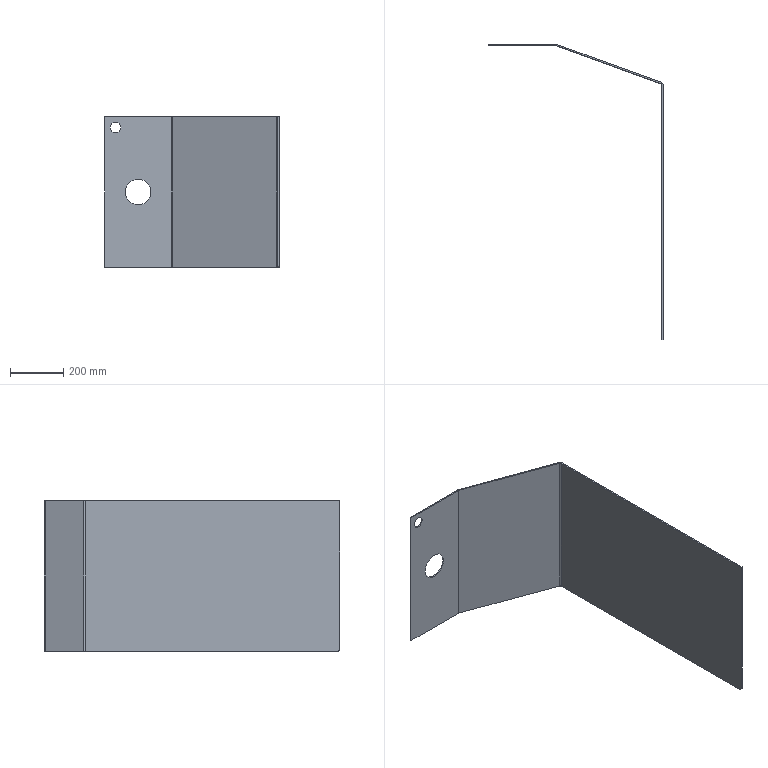Part | SolidWorks | features Fillet 1, FlatPattern 1, ICE 1, SMBaseFlange 1, SheetMetal 1, UnFold 1 | 1 solid | 27 faces | box 655 x 1110 x 565 mm | volume 4586470 mm3 | plane 18 | cylinder 9 | commonest cylinder face diameters 12 x2 22 x2 40 x2 97 x2 14 x1
STEP:
#1=CARTESIAN_POINT('',(125.,1105.,-48.5));
#2=VERTEX_POINT('',#1);
#3=CARTESIAN_POINT('',(125.,1105.,48.5));
#4=VERTEX_POINT('',#3);
#5=CARTESIAN_POINT('',(125.,1105.,0.));
#6=DIRECTION('',(0.,1.,0.));
#7=DIRECTION('',(0.,0.,1.));
#8=AXIS2_PLACEMENT_3D('',#5,#6,#7);
#9=CIRCLE('',#8,48.5);
#10=EDGE_CURVE('',#2,#4,#9,.T.);
#11=ORIENTED_EDGE('',*,*,#10,.F.);
#12=CARTESIAN_POINT('',(125.,1110.,-48.5));
#13=VERTEX_POINT('',#12);
#14=CARTESIAN_POINT('',(125.,0.,-48.5));
#15=DIRECTION('',(0.,1.,0.));
#16=VECTOR('',#15,1000.);
#17=LINE('',#14,#16);
#18=EDGE_CURVE('',#2,#13,#17,.T.);
#19=ORIENTED_EDGE('',*,*,#18,.T.);
#20=CARTESIAN_POINT('',(125.,1110.,48.5));
#21=VERTEX_POINT('',#20);
#22=CARTESIAN_POINT('',(125.,1110.,0.));
#23=DIRECTION('',(0.,1.,0.));
#24=DIRECTION('',(0.,0.,1.));
#25=AXIS2_PLACEMENT_3D('',#22,#23,#24);
#26=CIRCLE('',#25,48.5);
#27=EDGE_CURVE('',#13,#21,#26,.T.);
#28=ORIENTED_EDGE('',*,*,#27,.T.);
#29=CARTESIAN_POINT('',(125.,0.,48.5));
#30=DIRECTION('',(0.,1.,0.));
#31=VECTOR('',#30,1000.);
#32=LINE('',#29,#31);
#33=EDGE_CURVE('',#4,#21,#32,.T.);
#34=ORIENTED_EDGE('',*,*,#33,.F.);
#35=EDGE_LOOP('',(#11,#19,#28,#34));
#36=FACE_OUTER_BOUND('',#35,.T.);
#37=CARTESIAN_POINT('',(125.,0.,0.));
#38=DIRECTION('',(0.,1.,0.));
#39=DIRECTION('',(0.,0.,1.));
#40=AXIS2_PLACEMENT_3D('',#37,#38,#39);
#41=CYLINDRICAL_SURFACE('',#40,48.5);
#42=ADVANCED_FACE('',(#36),#41,.F.);
#43=CARTESIAN_POINT('',(40.,1105.,222.5));
#44=VERTEX_POINT('',#43);
#45=CARTESIAN_POINT('',(40.,1105.,262.5));
#46=VERTEX_POINT('',#45);
#47=CARTESIAN_POINT('',(40.,1105.,242.5));
#48=DIRECTION('',(0.,1.,0.));
#49=DIRECTION('',(0.,0.,1.));
#50=AXIS2_PLACEMENT_3D('',#47,#48,#49);
#51=CIRCLE('',#50,20.);
#52=EDGE_CURVE('',#44,#46,#51,.T.);
#53=ORIENTED_EDGE('',*,*,#52,.F.);
#54=CARTESIAN_POINT('',(40.,1110.,222.5));
#55=VERTEX_POINT('',#54);
#56=CARTESIAN_POINT('',(40.,0.,222.5));
#57=DIRECTION('',(0.,1.,0.));
#58=VECTOR('',#57,1000.);
#59=LINE('',#56,#58);
#60=EDGE_CURVE('',#44,#55,#59,.T.);
#61=ORIENTED_EDGE('',*,*,#60,.T.);
#62=CARTESIAN_POINT('',(40.,1110.,262.5));
#63=VERTEX_POINT('',#62);
#64=CARTESIAN_POINT('',(40.,1110.,242.5));
#65=DIRECTION('',(0.,1.,0.));
#66=DIRECTION('',(0.,0.,1.));
#67=AXIS2_PLACEMENT_3D('',#64,#65,#66);
#68=CIRCLE('',#67,20.);
#69=EDGE_CURVE('',#55,#63,#68,.T.);
#70=ORIENTED_EDGE('',*,*,#69,.T.);
#71=CARTESIAN_POINT('',(40.,0.,262.5));
#72=DIRECTION('',(0.,1.,0.));
#73=VECTOR('',#72,1000.);
#74=LINE('',#71,#73);
#75=EDGE_CURVE('',#46,#63,#74,.T.);
#76=ORIENTED_EDGE('',*,*,#75,.F.);
#77=EDGE_LOOP('',(#53,#61,#70,#76));
#78=FACE_OUTER_BOUND('',#77,.T.);
#79=CARTESIAN_POINT('',(40.,0.,242.5));
#80=DIRECTION('',(0.,1.,0.));
#81=DIRECTION('',(0.,0.,1.));
#82=AXIS2_PLACEMENT_3D('',#79,#80,#81);
#83=CYLINDRICAL_SURFACE('',#82,20.);
#84=ADVANCED_FACE('',(#78),#83,.F.);
#85=CARTESIAN_POINT('',(255.823,1109.337,282.5));
#86=VERTEX_POINT('',#85);
#87=CARTESIAN_POINT('',(254.113,1104.638,282.5));
#88=VERTEX_POINT('',#87);
#89=CARTESIAN_POINT('',(255.823,1109.337,282.5));
#90=DIRECTION('',(-0.342,-0.9397,0.));
#91=VECTOR('',#90,1000.);
#92=LINE('',#89,#91);
#93=EDGE_CURVE('',#86,#88,#92,.T.);
#94=ORIENTED_EDGE('',*,*,#93,.F.);
#95=CARTESIAN_POINT('',(252.06,1110.,282.5));
#96=VERTEX_POINT('',#95);
#97=CARTESIAN_POINT('',(252.06,1099.,282.5));
#98=DIRECTION('',(0.,0.,-1.));
#99=DIRECTION('',(1.,0.,0.));
#100=AXIS2_PLACEMENT_3D('',#97,#98,#99);
#101=CIRCLE('',#100,11.);
#102=EDGE_CURVE('',#96,#86,#101,.T.);
#103=ORIENTED_EDGE('',*,*,#102,.F.);
#104=CARTESIAN_POINT('',(252.06,1105.,282.5));
#105=VERTEX_POINT('',#104);
#106=CARTESIAN_POINT('',(252.06,1105.,282.5));
#107=DIRECTION('',(0.,1.,0.));
#108=VECTOR('',#107,1000.);
#109=LINE('',#106,#108);
#110=EDGE_CURVE('',#105,#96,#109,.T.);
#111=ORIENTED_EDGE('',*,*,#110,.F.);
#112=CARTESIAN_POINT('',(252.06,1099.,282.5));
#113=DIRECTION('',(0.,0.,-1.));
#114=DIRECTION('',(1.,0.,0.));
#115=AXIS2_PLACEMENT_3D('',#112,#113,#114);
#116=CIRCLE('',#115,6.);
#117=EDGE_CURVE('',#105,#88,#116,.T.);
#118=ORIENTED_EDGE('',*,*,#117,.T.);
#119=EDGE_LOOP('',(#94,#103,#111,#118));
#120=FACE_OUTER_BOUND('',#119,.T.);
#121=CARTESIAN_POINT('',(255.823,1109.337,282.5));
#122=DIRECTION('',(0.,0.,1.));
#123=DIRECTION('',(1.,0.,0.));
#124=AXIS2_PLACEMENT_3D('',#121,#122,#123);
#125=PLANE('',#124);
#126=ADVANCED_FACE('',(#120),#125,.T.);
#127=CARTESIAN_POINT('',(647.762,966.682,282.5));
#128=VERTEX_POINT('',#127);
#129=CARTESIAN_POINT('',(254.,1110.,282.5));
#130=DIRECTION('',(0.9397,-0.342,0.));
#131=VECTOR('',#130,1000.);
#132=LINE('',#129,#131);
#133=EDGE_CURVE('',#86,#128,#132,.T.);
#134=ORIENTED_EDGE('',*,*,#133,.F.);
#135=ORIENTED_EDGE('',*,*,#93,.T.);
#136=CARTESIAN_POINT('',(646.052,961.984,282.5));
#137=VERTEX_POINT('',#136);
#138=CARTESIAN_POINT('',(252.29,1105.302,282.5));
#139=DIRECTION('',(0.9397,-0.342,0.));
#140=VECTOR('',#139,1000.);
#141=LINE('',#138,#140);
#142=EDGE_CURVE('',#88,#137,#141,.T.);
#143=ORIENTED_EDGE('',*,*,#142,.T.);
#144=CARTESIAN_POINT('',(646.052,961.984,282.5));
#145=DIRECTION('',(0.342,0.9397,0.));
#146=VECTOR('',#145,1000.);
#147=LINE('',#144,#146);
#148=EDGE_CURVE('',#137,#128,#147,.T.);
#149=ORIENTED_EDGE('',*,*,#148,.T.);
#150=EDGE_LOOP('',(#134,#135,#143,#149));
#151=FACE_OUTER_BOUND('',#150,.T.);
#152=CARTESIAN_POINT('',(252.06,1105.,282.5));
#153=DIRECTION('',(0.,0.,1.));
#154=DIRECTION('',(1.,0.,0.));
#155=AXIS2_PLACEMENT_3D('',#152,#153,#154);
#156=PLANE('',#155);
#157=ADVANCED_FACE('',(#151),#156,.T.);
#158=CARTESIAN_POINT('',(252.06,1110.,-282.5));
#159=VERTEX_POINT('',#158);
#160=CARTESIAN_POINT('',(252.06,1105.,-282.5));
#161=VERTEX_POINT('',#160);
#162=CARTESIAN_POINT('',(252.06,1110.,-282.5));
#163=DIRECTION('',(0.,-1.,0.));
#164=VECTOR('',#163,1000.);
#165=LINE('',#162,#164);
#166=EDGE_CURVE('',#159,#161,#165,.T.);
#167=ORIENTED_EDGE('',*,*,#166,.F.);
#168=CARTESIAN_POINT('',(255.823,1109.337,-282.5));
#169=VERTEX_POINT('',#168);
#170=CARTESIAN_POINT('',(252.06,1099.,-282.5));
#171=DIRECTION('',(0.,0.,-1.));
#172=DIRECTION('',(1.,0.,0.));
#173=AXIS2_PLACEMENT_3D('',#170,#171,#172);
#174=CIRCLE('',#173,11.);
#175=EDGE_CURVE('',#159,#169,#174,.T.);
#176=ORIENTED_EDGE('',*,*,#175,.T.);
#177=CARTESIAN_POINT('',(254.113,1104.638,-282.5));
#178=VERTEX_POINT('',#177);
#179=CARTESIAN_POINT('',(254.113,1104.638,-282.5));
#180=DIRECTION('',(0.342,0.9397,0.));
#181=VECTOR('',#180,1000.);
#182=LINE('',#179,#181);
#183=EDGE_CURVE('',#178,#169,#182,.T.);
#184=ORIENTED_EDGE('',*,*,#183,.F.);
#185=CARTESIAN_POINT('',(252.06,1099.,-282.5));
#186=DIRECTION('',(0.,0.,-1.));
#187=DIRECTION('',(1.,0.,0.));
#188=AXIS2_PLACEMENT_3D('',#185,#186,#187);
#189=CIRCLE('',#188,6.);
#190=EDGE_CURVE('',#161,#178,#189,.T.);
#191=ORIENTED_EDGE('',*,*,#190,.F.);
#192=EDGE_LOOP('',(#167,#176,#184,#191));
#193=FACE_OUTER_BOUND('',#192,.T.);
#194=CARTESIAN_POINT('',(252.06,1110.,-282.5));
#195=DIRECTION('',(0.,0.,-1.));
#196=DIRECTION('',(-1.,0.,0.));
#197=AXIS2_PLACEMENT_3D('',#194,#195,#196);
#198=PLANE('',#197);
#199=ADVANCED_FACE('',(#193),#198,.T.);
#200=CARTESIAN_POINT('',(0.,1110.,-282.5));
#201=VERTEX_POINT('',#200);
#202=CARTESIAN_POINT('',(0.,1110.,-282.5));
#203=DIRECTION('',(1.,0.,0.));
#204=VECTOR('',#203,1000.);
#205=LINE('',#202,#204);
#206=EDGE_CURVE('',#201,#159,#205,.T.);
#207=ORIENTED_EDGE('',*,*,#206,.T.);
#208=ORIENTED_EDGE('',*,*,#166,.T.);
#209=CARTESIAN_POINT('',(0.,1105.,-282.5));
#210=VERTEX_POINT('',#209);
#211=CARTESIAN_POINT('',(0.,1105.,-282.5));
#212=DIRECTION('',(1.,0.,0.));
#213=VECTOR('',#212,1000.);
#214=LINE('',#211,#213);
#215=EDGE_CURVE('',#210,#161,#214,.T.);
#216=ORIENTED_EDGE('',*,*,#215,.F.);
#217=CARTESIAN_POINT('',(0.,1105.,-282.5));
#218=DIRECTION('',(0.,1.,0.));
#219=VECTOR('',#218,1000.);
#220=LINE('',#217,#219);
#221=EDGE_CURVE('',#210,#201,#220,.T.);
#222=ORIENTED_EDGE('',*,*,#221,.T.);
#223=EDGE_LOOP('',(#207,#208,#216,#222));
#224=FACE_OUTER_BOUND('',#223,.T.);
#225=CARTESIAN_POINT('',(254.113,1104.638,-282.5));
#226=DIRECTION('',(0.,0.,-1.));
#227=DIRECTION('',(-1.,0.,0.));
#228=AXIS2_PLACEMENT_3D('',#225,#226,#227);
#229=PLANE('',#228);
#230=ADVANCED_FACE('',(#224),#229,.T.);
#231=CARTESIAN_POINT('',(655.,956.346,282.5));
#232=VERTEX_POINT('',#231);
#233=CARTESIAN_POINT('',(650.,956.346,282.5));
#234=VERTEX_POINT('',#233);
#235=CARTESIAN_POINT('',(655.,956.346,282.5));
#236=DIRECTION('',(-1.,0.,0.));
#237=VECTOR('',#236,1000.);
#238=LINE('',#235,#237);
#239=EDGE_CURVE('',#232,#234,#238,.T.);
#240=ORIENTED_EDGE('',*,*,#239,.F.);
#241=CARTESIAN_POINT('',(644.,956.346,282.5));
#242=DIRECTION('',(0.,0.,-1.));
#243=DIRECTION('',(1.,0.,0.));
#244=AXIS2_PLACEMENT_3D('',#241,#242,#243);
#245=CIRCLE('',#244,11.);
#246=EDGE_CURVE('',#128,#232,#245,.T.);
#247=ORIENTED_EDGE('',*,*,#246,.F.);
#248=ORIENTED_EDGE('',*,*,#148,.F.);
#249=CARTESIAN_POINT('',(644.,956.346,282.5));
#250=DIRECTION('',(0.,0.,-1.));
#251=DIRECTION('',(1.,0.,0.));
#252=AXIS2_PLACEMENT_3D('',#249,#250,#251);
#253=CIRCLE('',#252,6.);
#254=EDGE_CURVE('',#137,#234,#253,.T.);
#255=ORIENTED_EDGE('',*,*,#254,.T.);
#256=EDGE_LOOP('',(#240,#247,#248,#255));
#257=FACE_OUTER_BOUND('',#256,.T.);
#258=CARTESIAN_POINT('',(655.,956.346,282.5));
#259=DIRECTION('',(0.,0.,1.));
#260=DIRECTION('',(1.,0.,0.));
#261=AXIS2_PLACEMENT_3D('',#258,#259,#260);
#262=PLANE('',#261);
#263=ADVANCED_FACE('',(#257),#262,.T.);
#264=CARTESIAN_POINT('',(655.,0.,282.5));
#265=VERTEX_POINT('',#264);
#266=CARTESIAN_POINT('',(655.,964.048,282.5));
#267=DIRECTION('',(0.,-1.,0.));
#268=VECTOR('',#267,1000.);
#269=LINE('',#266,#268);
#270=EDGE_CURVE('',#232,#265,#269,.T.);
#271=ORIENTED_EDGE('',*,*,#270,.F.);
#272=ORIENTED_EDGE('',*,*,#239,.T.);
#273=CARTESIAN_POINT('',(650.,0.,282.5));
#274=VERTEX_POINT('',#273);
#275=CARTESIAN_POINT('',(650.,964.048,282.5));
#276=DIRECTION('',(0.,-1.,0.));
#277=VECTOR('',#276,1000.);
#278=LINE('',#275,#277);
#279=EDGE_CURVE('',#234,#274,#278,.T.);
#280=ORIENTED_EDGE('',*,*,#279,.T.);
#281=CARTESIAN_POINT('',(655.,0.,282.5));
#282=DIRECTION('',(-1.,0.,0.));
#283=VECTOR('',#282,1000.);
#284=LINE('',#281,#283);
#285=EDGE_CURVE('',#265,#274,#284,.T.);
#286=ORIENTED_EDGE('',*,*,#285,.F.);
#287=EDGE_LOOP('',(#271,#272,#280,#286));
#288=FACE_OUTER_BOUND('',#287,.T.);
#289=CARTESIAN_POINT('',(646.052,961.984,282.5));
#290=DIRECTION('',(0.,0.,1.));
#291=DIRECTION('',(1.,0.,0.));
#292=AXIS2_PLACEMENT_3D('',#289,#290,#291);
#293=PLANE('',#292);
#294=ADVANCED_FACE('',(#288),#293,.T.);
#295=CARTESIAN_POINT('',(647.762,966.682,-282.5));
#296=VERTEX_POINT('',#295);
#297=CARTESIAN_POINT('',(646.052,961.984,-282.5));
#298=VERTEX_POINT('',#297);
#299=CARTESIAN_POINT('',(647.762,966.682,-282.5));
#300=DIRECTION('',(-0.342,-0.9397,0.));
#301=VECTOR('',#300,1000.);
#302=LINE('',#299,#301);
#303=EDGE_CURVE('',#296,#298,#302,.T.);
#304=ORIENTED_EDGE('',*,*,#303,.F.);
#305=CARTESIAN_POINT('',(655.,956.346,-282.5));
#306=VERTEX_POINT('',#305);
#307=CARTESIAN_POINT('',(644.,956.346,-282.5));
#308=DIRECTION('',(0.,0.,-1.));
#309=DIRECTION('',(1.,0.,0.));
#310=AXIS2_PLACEMENT_3D('',#307,#308,#309);
#311=CIRCLE('',#310,11.);
#312=EDGE_CURVE('',#296,#306,#311,.T.);
#313=ORIENTED_EDGE('',*,*,#312,.T.);
#314=CARTESIAN_POINT('',(650.,956.346,-282.5));
#315=VERTEX_POINT('',#314);
#316=CARTESIAN_POINT('',(650.,956.346,-282.5));
#317=DIRECTION('',(1.,0.,0.));
#318=VECTOR('',#317,1000.);
#319=LINE('',#316,#318);
#320=EDGE_CURVE('',#315,#306,#319,.T.);
#321=ORIENTED_EDGE('',*,*,#320,.F.);
#322=CARTESIAN_POINT('',(644.,956.346,-282.5));
#323=DIRECTION('',(0.,0.,-1.));
#324=DIRECTION('',(1.,0.,0.));
#325=AXIS2_PLACEMENT_3D('',#322,#323,#324);
#326=CIRCLE('',#325,6.);
#327=EDGE_CURVE('',#298,#315,#326,.T.);
#328=ORIENTED_EDGE('',*,*,#327,.F.);
#329=EDGE_LOOP('',(#304,#313,#321,#328));
#330=FACE_OUTER_BOUND('',#329,.T.);
#331=CARTESIAN_POINT('',(647.762,966.682,-282.5));
#332=DIRECTION('',(0.,0.,-1.));
#333=DIRECTION('',(-1.,0.,0.));
#334=AXIS2_PLACEMENT_3D('',#331,#332,#333);
#335=PLANE('',#334);
#336=ADVANCED_FACE('',(#330),#335,.T.);
#337=CARTESIAN_POINT('',(254.,1110.,-282.5));
#338=DIRECTION('',(0.9397,-0.342,0.));
#339=VECTOR('',#338,1000.);
#340=LINE('',#337,#339);
#341=EDGE_CURVE('',#169,#296,#340,.T.);
#342=ORIENTED_EDGE('',*,*,#341,.T.);
#343=ORIENTED_EDGE('',*,*,#303,.T.);
#344=CARTESIAN_POINT('',(252.29,1105.302,-282.5));
#345=DIRECTION('',(0.9397,-0.342,0.));
#346=VECTOR('',#345,1000.);
#347=LINE('',#344,#346);
#348=EDGE_CURVE('',#178,#298,#347,.T.);
#349=ORIENTED_EDGE('',*,*,#348,.F.);
#350=ORIENTED_EDGE('',*,*,#183,.T.);
#351=EDGE_LOOP('',(#342,#343,#349,#350));
#352=FACE_OUTER_BOUND('',#351,.T.);
#353=CARTESIAN_POINT('',(650.,956.346,-282.5));
#354=DIRECTION('',(0.,0.,-1.));
#355=DIRECTION('',(-1.,0.,0.));
#356=AXIS2_PLACEMENT_3D('',#353,#354,#355);
#357=PLANE('',#356);
#358=ADVANCED_FACE('',(#352),#357,.T.);
#359=CARTESIAN_POINT('',(650.,7.,-282.5));
#360=VERTEX_POINT('',#359);
#361=CARTESIAN_POINT('',(650.,964.048,-282.5));
#362=DIRECTION('',(0.,-1.,0.));
#363=VECTOR('',#362,1000.);
#364=LINE('',#361,#363);
#365=EDGE_CURVE('',#315,#360,#364,.T.);
#366=ORIENTED_EDGE('',*,*,#365,.T.);
#367=CARTESIAN_POINT('',(650.,0.,-275.5));
#368=VERTEX_POINT('',#367);
#369=CARTESIAN_POINT('',(650.,7.,-275.5));
#370=DIRECTION('',(-1.,0.,0.));
#371=DIRECTION('',(0.,1.,0.));
#372=AXIS2_PLACEMENT_3D('',#369,#370,#371);
#373=CIRCLE('',#372,7.);
#374=EDGE_CURVE('',#360,#368,#373,.T.);
#375=ORIENTED_EDGE('',*,*,#374,.T.);
#376=CARTESIAN_POINT('',(650.,0.,282.5));
#377=DIRECTION('',(0.,0.,-1.));
#378=VECTOR('',#377,1000.);
#379=LINE('',#376,#378);
#380=EDGE_CURVE('',#274,#368,#379,.T.);
#381=ORIENTED_EDGE('',*,*,#380,.F.);
#382=ORIENTED_EDGE('',*,*,#279,.F.);
#383=CARTESIAN_POINT('',(650.,956.346,282.5));
#384=DIRECTION('',(0.,0.,-1.));
#385=VECTOR('',#384,1000.);
#386=LINE('',#383,#385);
#387=EDGE_CURVE('',#234,#315,#386,.T.);
#388=ORIENTED_EDGE('',*,*,#387,.T.);
#389=EDGE_LOOP('',(#366,#375,#381,#382,#388));
#390=FACE_OUTER_BOUND('',#389,.T.);
#391=CARTESIAN_POINT('',(650.,964.048,282.5));
#392=DIRECTION('',(1.,0.,0.));
#393=DIRECTION('',(0.,1.,0.));
#394=AXIS2_PLACEMENT_3D('',#391,#392,#393);
#395=PLANE('',#394);
#396=ADVANCED_FACE('',(#390),#395,.F.);
#397=ORIENTED_EDGE('',*,*,#380,.T.);
#398=CARTESIAN_POINT('',(655.,0.,-275.5));
#399=VERTEX_POINT('',#398);
#400=CARTESIAN_POINT('',(655.,0.,-275.5));
#401=DIRECTION('',(1.,0.,0.));
#402=VECTOR('',#401,1000.);
#403=LINE('',#400,#402);
#404=EDGE_CURVE('',#368,#399,#403,.T.);
#405=ORIENTED_EDGE('',*,*,#404,.T.);
#406=CARTESIAN_POINT('',(655.,0.,282.5));
#407=DIRECTION('',(0.,0.,-1.));
#408=VECTOR('',#407,1000.);
#409=LINE('',#406,#408);
#410=EDGE_CURVE('',#265,#399,#409,.T.);
#411=ORIENTED_EDGE('',*,*,#410,.F.);
#412=ORIENTED_EDGE('',*,*,#285,.T.);
#413=EDGE_LOOP('',(#397,#405,#411,#412));
#414=FACE_OUTER_BOUND('',#413,.T.);
#415=CARTESIAN_POINT('',(655.,0.,282.5));
#416=DIRECTION('',(0.,-1.,0.));
#417=DIRECTION('',(0.,0.,-1.));
#418=AXIS2_PLACEMENT_3D('',#415,#416,#417);
#419=PLANE('',#418);
#420=ADVANCED_FACE('',(#414),#419,.T.);
#421=ORIENTED_EDGE('',*,*,#410,.T.);
#422=CARTESIAN_POINT('',(655.,7.,-282.5));
#423=VERTEX_POINT('',#422);
#424=CARTESIAN_POINT('',(655.,7.,-275.5));
#425=DIRECTION('',(1.,0.,0.));
#426=DIRECTION('',(0.,1.,0.));
#427=AXIS2_PLACEMENT_3D('',#424,#425,#426);
#428=CIRCLE('',#427,7.);
#429=EDGE_CURVE('',#399,#423,#428,.T.);
#430=ORIENTED_EDGE('',*,*,#429,.T.);
#431=CARTESIAN_POINT('',(655.,964.048,-282.5));
#432=DIRECTION('',(0.,-1.,0.));
#433=VECTOR('',#432,1000.);
#434=LINE('',#431,#433);
#435=EDGE_CURVE('',#306,#423,#434,.T.);
#436=ORIENTED_EDGE('',*,*,#435,.F.);
#437=CARTESIAN_POINT('',(655.,956.346,282.5));
#438=DIRECTION('',(0.,0.,-1.));
#439=VECTOR('',#438,1000.);
#440=LINE('',#437,#439);
#441=EDGE_CURVE('',#232,#306,#440,.T.);
#442=ORIENTED_EDGE('',*,*,#441,.F.);
#443=ORIENTED_EDGE('',*,*,#270,.T.);
#444=EDGE_LOOP('',(#421,#430,#436,#442,#443));
#445=FACE_OUTER_BOUND('',#444,.T.);
#446=CARTESIAN_POINT('',(655.,964.048,282.5));
#447=DIRECTION('',(1.,0.,0.));
#448=DIRECTION('',(0.,1.,0.));
#449=AXIS2_PLACEMENT_3D('',#446,#447,#448);
#450=PLANE('',#449);
#451=ADVANCED_FACE('',(#445),#450,.T.);
#452=ORIENTED_EDGE('',*,*,#312,.F.);
#453=CARTESIAN_POINT('',(647.762,966.682,282.5));
#454=DIRECTION('',(0.,0.,-1.));
#455=VECTOR('',#454,1000.);
#456=LINE('',#453,#455);
#457=EDGE_CURVE('',#128,#296,#456,.T.);
#458=ORIENTED_EDGE('',*,*,#457,.F.);
#459=ORIENTED_EDGE('',*,*,#246,.T.);
#460=ORIENTED_EDGE('',*,*,#441,.T.);
#461=EDGE_LOOP('',(#452,#458,#459,#460));
#462=FACE_OUTER_BOUND('',#461,.T.);
#463=CARTESIAN_POINT('',(644.,956.346,282.5));
#464=DIRECTION('',(0.,0.,-1.));
#465=DIRECTION('',(-1.,0.,0.));
#466=AXIS2_PLACEMENT_3D('',#463,#464,#465);
#467=CYLINDRICAL_SURFACE('',#466,11.);
#468=ADVANCED_FACE('',(#462),#467,.T.);
#469=ORIENTED_EDGE('',*,*,#341,.F.);
#470=CARTESIAN_POINT('',(255.823,1109.337,282.5));
#471=DIRECTION('',(0.,0.,-1.));
#472=VECTOR('',#471,1000.);
#473=LINE('',#470,#472);
#474=EDGE_CURVE('',#86,#169,#473,.T.);
#475=ORIENTED_EDGE('',*,*,#474,.F.);
#476=ORIENTED_EDGE('',*,*,#133,.T.);
#477=ORIENTED_EDGE('',*,*,#457,.T.);
#478=EDGE_LOOP('',(#469,#475,#476,#477));
#479=FACE_OUTER_BOUND('',#478,.T.);
#480=CARTESIAN_POINT('',(254.,1110.,282.5));
#481=DIRECTION('',(0.342,0.9397,0.));
#482=DIRECTION('',(-0.9397,0.342,0.));
#483=AXIS2_PLACEMENT_3D('',#480,#481,#482);
#484=PLANE('',#483);
#485=ADVANCED_FACE('',(#479),#484,.T.);
#486=ORIENTED_EDGE('',*,*,#175,.F.);
#487=CARTESIAN_POINT('',(252.06,1110.,282.5));
#488=DIRECTION('',(0.,0.,-1.));
#489=VECTOR('',#488,1000.);
#490=LINE('',#487,#489);
#491=EDGE_CURVE('',#96,#159,#490,.T.);
#492=ORIENTED_EDGE('',*,*,#491,.F.);
#493=ORIENTED_EDGE('',*,*,#102,.T.);
#494=ORIENTED_EDGE('',*,*,#474,.T.);
#495=EDGE_LOOP('',(#486,#492,#493,#494));
#496=FACE_OUTER_BOUND('',#495,.T.);
#497=CARTESIAN_POINT('',(252.06,1099.,282.5));
#498=DIRECTION('',(0.,0.,-1.));
#499=DIRECTION('',(-1.,0.,0.));
#500=AXIS2_PLACEMENT_3D('',#497,#498,#499);
#501=CYLINDRICAL_SURFACE('',#500,11.);
#502=ADVANCED_FACE('',(#496),#501,.T.);
#503=CARTESIAN_POINT('',(125.,1110.,0.));
#504=DIRECTION('',(0.,1.,0.));
#505=DIRECTION('',(0.,0.,1.));
#506=AXIS2_PLACEMENT_3D('',#503,#504,#505);
#507=CIRCLE('',#506,48.5);
#508=EDGE_CURVE('',#21,#13,#507,.T.);
#509=ORIENTED_EDGE('',*,*,#508,.F.);
#510=ORIENTED_EDGE('',*,*,#27,.F.);
#511=EDGE_LOOP('',(#509,#510));
#512=FACE_BOUND('',#511,.T.);
#513=CARTESIAN_POINT('',(40.,1110.,242.5));
#514=DIRECTION('',(0.,1.,0.));
#515=DIRECTION('',(0.,0.,1.));
#516=AXIS2_PLACEMENT_3D('',#513,#514,#515);
#517=CIRCLE('',#516,20.);
#518=EDGE_CURVE('',#63,#55,#517,.T.);
#519=ORIENTED_EDGE('',*,*,#518,.F.);
#520=ORIENTED_EDGE('',*,*,#69,.F.);
#521=EDGE_LOOP('',(#519,#520));
#522=FACE_BOUND('',#521,.T.);
#523=ORIENTED_EDGE('',*,*,#206,.F.);
#524=CARTESIAN_POINT('',(0.,1110.,282.5));
#525=VERTEX_POINT('',#524);
#526=CARTESIAN_POINT('',(0.,1110.,282.5));
#527=DIRECTION('',(0.,0.,-1.));
#528=VECTOR('',#527,1000.);
#529=LINE('',#526,#528);
#530=EDGE_CURVE('',#525,#201,#529,.T.);
#531=ORIENTED_EDGE('',*,*,#530,.F.);
#532=CARTESIAN_POINT('',(0.,1110.,282.5));
#533=DIRECTION('',(1.,0.,0.));
#534=VECTOR('',#533,1000.);
#535=LINE('',#532,#534);
#536=EDGE_CURVE('',#525,#96,#535,.T.);
#537=ORIENTED_EDGE('',*,*,#536,.T.);
#538=ORIENTED_EDGE('',*,*,#491,.T.);
#539=EDGE_LOOP('',(#523,#531,#537,#538));
#540=FACE_OUTER_BOUND('',#539,.T.);
#541=CARTESIAN_POINT('',(0.,1110.,282.5));
#542=DIRECTION('',(0.,1.,0.));
#543=DIRECTION('',(0.,0.,1.));
#544=AXIS2_PLACEMENT_3D('',#541,#542,#543);
#545=PLANE('',#544);
#546=ADVANCED_FACE('',(#512,#522,#540),#545,.T.);
#547=ORIENTED_EDGE('',*,*,#221,.F.);
#548=CARTESIAN_POINT('',(0.,1105.,282.5));
#549=VERTEX_POINT('',#548);
#550=CARTESIAN_POINT('',(0.,1105.,282.5));
#551=DIRECTION('',(0.,0.,-1.));
#552=VECTOR('',#551,1000.);
#553=LINE('',#550,#552);
#554=EDGE_CURVE('',#549,#210,#553,.T.);
#555=ORIENTED_EDGE('',*,*,#554,.F.);
#556=CARTESIAN_POINT('',(0.,1105.,282.5));
#557=DIRECTION('',(0.,1.,0.));
#558=VECTOR('',#557,1000.);
#559=LINE('',#556,#558);
#560=EDGE_CURVE('',#549,#525,#559,.T.);
#561=ORIENTED_EDGE('',*,*,#560,.T.);
#562=ORIENTED_EDGE('',*,*,#530,.T.);
#563=EDGE_LOOP('',(#547,#555,#561,#562));
#564=FACE_OUTER_BOUND('',#563,.T.);
#565=CARTESIAN_POINT('',(0.,1105.,282.5));
#566=DIRECTION('',(-1.,0.,0.));
#567=DIRECTION('',(0.,0.,1.));
#568=AXIS2_PLACEMENT_3D('',#565,#566,#567);
#569=PLANE('',#568);
#570=ADVANCED_FACE('',(#564),#569,.T.);
#571=CARTESIAN_POINT('',(125.,1105.,0.));
#572=DIRECTION('',(0.,1.,0.));
#573=DIRECTION('',(0.,0.,1.));
#574=AXIS2_PLACEMENT_3D('',#571,#572,#573);
#575=CIRCLE('',#574,48.5);
#576=EDGE_CURVE('',#4,#2,#575,.T.);
#577=ORIENTED_EDGE('',*,*,#576,.T.);
#578=ORIENTED_EDGE('',*,*,#10,.T.);
#579=EDGE_LOOP('',(#577,#578));
#580=FACE_BOUND('',#579,.T.);
#581=CARTESIAN_POINT('',(40.,1105.,242.5));
#582=DIRECTION('',(0.,1.,0.));
#583=DIRECTION('',(0.,0.,1.));
#584=AXIS2_PLACEMENT_3D('',#581,#582,#583);
#585=CIRCLE('',#584,20.);
#586=EDGE_CURVE('',#46,#44,#585,.T.);
#587=ORIENTED_EDGE('',*,*,#586,.T.);
#588=ORIENTED_EDGE('',*,*,#52,.T.);
#589=EDGE_LOOP('',(#587,#588));
#590=FACE_BOUND('',#589,.T.);
#591=ORIENTED_EDGE('',*,*,#215,.T.);
#592=CARTESIAN_POINT('',(252.06,1105.,282.5));
#593=DIRECTION('',(0.,0.,-1.));
#594=VECTOR('',#593,1000.);
#595=LINE('',#592,#594);
#596=EDGE_CURVE('',#105,#161,#595,.T.);
#597=ORIENTED_EDGE('',*,*,#596,.F.);
#598=CARTESIAN_POINT('',(0.,1105.,282.5));
#599=DIRECTION('',(1.,0.,0.));
#600=VECTOR('',#599,1000.);
#601=LINE('',#598,#600);
#602=EDGE_CURVE('',#549,#105,#601,.T.);
#603=ORIENTED_EDGE('',*,*,#602,.F.);
#604=ORIENTED_EDGE('',*,*,#554,.T.);
#605=EDGE_LOOP('',(#591,#597,#603,#604));
#606=FACE_OUTER_BOUND('',#605,.T.);
#607=CARTESIAN_POINT('',(0.,1105.,282.5));
#608=DIRECTION('',(0.,1.,0.));
#609=DIRECTION('',(0.,0.,1.));
#610=AXIS2_PLACEMENT_3D('',#607,#608,#609);
#611=PLANE('',#610);
#612=ADVANCED_FACE('',(#580,#590,#606),#611,.F.);
#613=ORIENTED_EDGE('',*,*,#190,.T.);
#614=CARTESIAN_POINT('',(254.113,1104.638,282.5));
#615=DIRECTION('',(0.,0.,-1.));
#616=VECTOR('',#615,1000.);
#617=LINE('',#614,#616);
#618=EDGE_CURVE('',#88,#178,#617,.T.);
#619=ORIENTED_EDGE('',*,*,#618,.F.);
#620=ORIENTED_EDGE('',*,*,#117,.F.);
#621=ORIENTED_EDGE('',*,*,#596,.T.);
#622=EDGE_LOOP('',(#613,#619,#620,#621));
#623=FACE_OUTER_BOUND('',#622,.T.);
#624=CARTESIAN_POINT('',(252.06,1099.,282.5));
#625=DIRECTION('',(0.,0.,-1.));
#626=DIRECTION('',(-1.,0.,0.));
#627=AXIS2_PLACEMENT_3D('',#624,#625,#626);
#628=CYLINDRICAL_SURFACE('',#627,6.);
#629=ADVANCED_FACE('',(#623),#628,.F.);
#630=ORIENTED_EDGE('',*,*,#348,.T.);
#631=CARTESIAN_POINT('',(646.052,961.984,282.5));
#632=DIRECTION('',(0.,0.,-1.));
#633=VECTOR('',#632,1000.);
#634=LINE('',#631,#633);
#635=EDGE_CURVE('',#137,#298,#634,.T.);
#636=ORIENTED_EDGE('',*,*,#635,.F.);
#637=ORIENTED_EDGE('',*,*,#142,.F.);
#638=ORIENTED_EDGE('',*,*,#618,.T.);
#639=EDGE_LOOP('',(#630,#636,#637,#638));
#640=FACE_OUTER_BOUND('',#639,.T.);
#641=CARTESIAN_POINT('',(252.29,1105.302,282.5));
#642=DIRECTION('',(0.342,0.9397,0.));
#643=DIRECTION('',(-0.9397,0.342,0.));
#644=AXIS2_PLACEMENT_3D('',#641,#642,#643);
#645=PLANE('',#644);
#646=ADVANCED_FACE('',(#640),#645,.F.);
#647=ORIENTED_EDGE('',*,*,#327,.T.);
#648=ORIENTED_EDGE('',*,*,#387,.F.);
#649=ORIENTED_EDGE('',*,*,#254,.F.);
#650=ORIENTED_EDGE('',*,*,#635,.T.);
#651=EDGE_LOOP('',(#647,#648,#649,#650));
#652=FACE_OUTER_BOUND('',#651,.T.);
#653=CARTESIAN_POINT('',(644.,956.346,282.5));
#654=DIRECTION('',(0.,0.,-1.));
#655=DIRECTION('',(-1.,0.,0.));
#656=AXIS2_PLACEMENT_3D('',#653,#654,#655);
#657=CYLINDRICAL_SURFACE('',#656,6.);
#658=ADVANCED_FACE('',(#652),#657,.F.);
#659=ORIENTED_EDGE('',*,*,#602,.T.);
#660=ORIENTED_EDGE('',*,*,#110,.T.);
#661=ORIENTED_EDGE('',*,*,#536,.F.);
#662=ORIENTED_EDGE('',*,*,#560,.F.);
#663=EDGE_LOOP('',(#659,#660,#661,#662));
#664=FACE_OUTER_BOUND('',#663,.T.);
#665=CARTESIAN_POINT('',(644.,956.346,282.5));
#666=DIRECTION('',(0.,0.,1.));
#667=DIRECTION('',(1.,0.,0.));
#668=AXIS2_PLACEMENT_3D('',#665,#666,#667);
#669=PLANE('',#668);
#670=ADVANCED_FACE('',(#664),#669,.T.);
#671=ORIENTED_EDGE('',*,*,#435,.T.);
#672=CARTESIAN_POINT('',(650.,7.,-282.5));
#673=DIRECTION('',(-1.,0.,0.));
#674=VECTOR('',#673,1000.);
#675=LINE('',#672,#674);
#676=EDGE_CURVE('',#423,#360,#675,.T.);
#677=ORIENTED_EDGE('',*,*,#676,.T.);
#678=ORIENTED_EDGE('',*,*,#365,.F.);
#679=ORIENTED_EDGE('',*,*,#320,.T.);
#680=EDGE_LOOP('',(#671,#677,#678,#679));
#681=FACE_OUTER_BOUND('',#680,.T.);
#682=CARTESIAN_POINT('',(644.,956.346,-282.5));
#683=DIRECTION('',(0.,0.,1.));
#684=DIRECTION('',(1.,0.,0.));
#685=AXIS2_PLACEMENT_3D('',#682,#683,#684);
#686=PLANE('',#685);
#687=ADVANCED_FACE('',(#681),#686,.F.);
#688=ORIENTED_EDGE('',*,*,#60,.F.);
#689=ORIENTED_EDGE('',*,*,#586,.F.);
#690=ORIENTED_EDGE('',*,*,#75,.T.);
#691=ORIENTED_EDGE('',*,*,#518,.T.);
#692=EDGE_LOOP('',(#688,#689,#690,#691));
#693=FACE_OUTER_BOUND('',#692,.T.);
#694=CARTESIAN_POINT('',(40.,0.,242.5));
#695=DIRECTION('',(0.,1.,0.));
#696=DIRECTION('',(0.,0.,1.));
#697=AXIS2_PLACEMENT_3D('',#694,#695,#696);
#698=CYLINDRICAL_SURFACE('',#697,20.);
#699=ADVANCED_FACE('',(#693),#698,.F.);
#700=ORIENTED_EDGE('',*,*,#18,.F.);
#701=ORIENTED_EDGE('',*,*,#576,.F.);
#702=ORIENTED_EDGE('',*,*,#33,.T.);
#703=ORIENTED_EDGE('',*,*,#508,.T.);
#704=EDGE_LOOP('',(#700,#701,#702,#703));
#705=FACE_OUTER_BOUND('',#704,.T.);
#706=CARTESIAN_POINT('',(125.,0.,0.));
#707=DIRECTION('',(0.,1.,0.));
#708=DIRECTION('',(0.,0.,1.));
#709=AXIS2_PLACEMENT_3D('',#706,#707,#708);
#710=CYLINDRICAL_SURFACE('',#709,48.5);
#711=ADVANCED_FACE('',(#705),#710,.F.);
#712=ORIENTED_EDGE('',*,*,#429,.F.);
#713=ORIENTED_EDGE('',*,*,#404,.F.);
#714=ORIENTED_EDGE('',*,*,#374,.F.);
#715=ORIENTED_EDGE('',*,*,#676,.F.);
#716=EDGE_LOOP('',(#712,#713,#714,#715));
#717=FACE_OUTER_BOUND('',#716,.T.);
#718=CARTESIAN_POINT('',(644.,7.,-275.5));
#719=DIRECTION('',(1.,0.,0.));
#720=DIRECTION('',(0.,0.,-1.));
#721=AXIS2_PLACEMENT_3D('',#718,#719,#720);
#722=CYLINDRICAL_SURFACE('',#721,7.);
#723=ADVANCED_FACE('',(#717),#722,.T.);
#724=CLOSED_SHELL('',(#42,#84,#126,#157,#199,#230,#263,#294,#336,#358,#396,#420,#451,#468,#485,#502,#546,#570,#612,#629,#646,#658,#670,#687,#699,#711,#723));
#725=MANIFOLD_SOLID_BREP('',#724);
#726=CARTESIAN_POINT('',(0.,0.,0.));
#727=DIRECTION('',(0.,0.,1.));
#728=DIRECTION('',(1.,0.,0.));
#729=AXIS2_PLACEMENT_3D('',#726,#727,#728);
#730=(LENGTH_UNIT()NAMED_UNIT(*)SI_UNIT(.MILLI.,.METRE.));
#731=UNCERTAINTY_MEASURE_WITH_UNIT(LENGTH_MEASURE(0.00001),#730,'','');
#732=(NAMED_UNIT(*)PLANE_ANGLE_UNIT()SI_UNIT($,.RADIAN.));
#733=(NAMED_UNIT(*)SI_UNIT($,.STERADIAN.)SOLID_ANGLE_UNIT());
#734=(GEOMETRIC_REPRESENTATION_CONTEXT(3)GLOBAL_UNCERTAINTY_ASSIGNED_CONTEXT((#731))GLOBAL_UNIT_ASSIGNED_CONTEXT((#730,#732,#733))REPRESENTATION_CONTEXT('',''));
#735=ADVANCED_BREP_SHAPE_REPRESENTATION('',(#725,#729),#734);